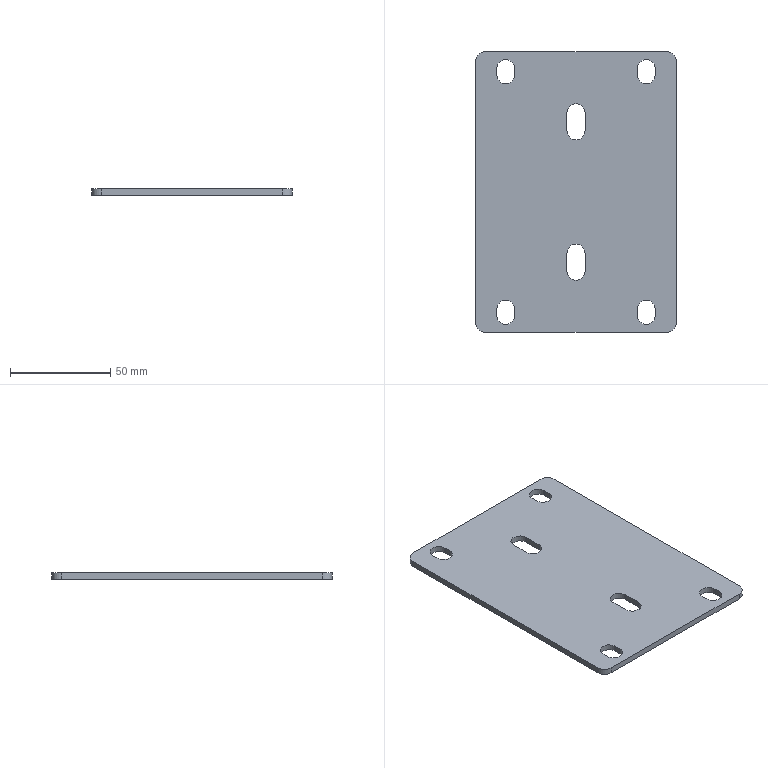Part | STEP file | 5091503M | 1 solid | 34 faces | box 100 x 140 x 3 mm | volume 39981 mm3 | plane 18 | cylinder 16 | commonest cylinder face diameters 9 x12 10 x4